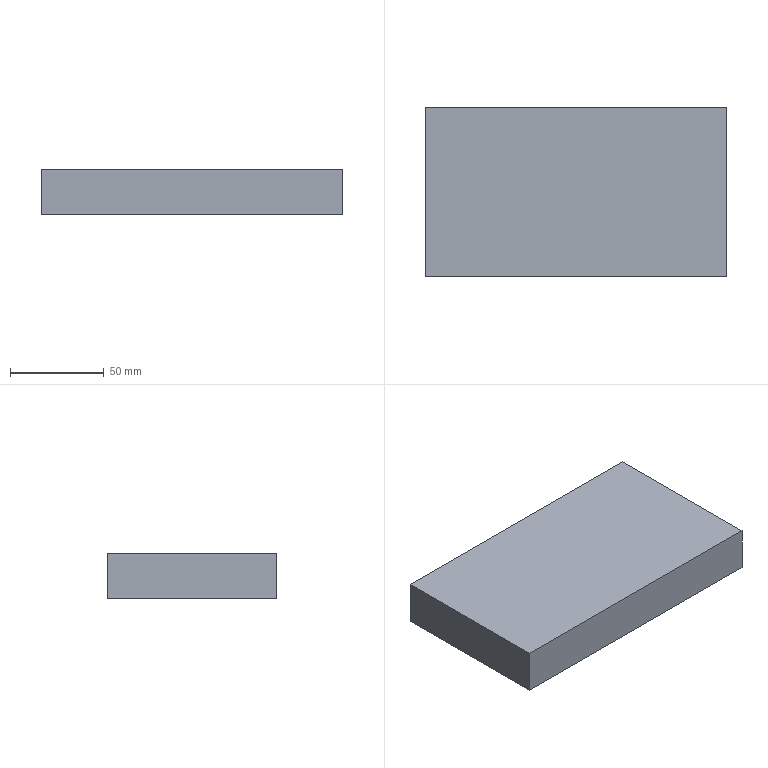Part | STEP file | 435_id754_x_t | 1 solid | 6 faces | box 160 x 90 x 24 mm | volume 345600 mm3 | plane 6
STEP:
#1=CARTESIAN_POINT('',(0.,0.,0.));
#2=DIRECTION('',(0.,0.,1.));
#3=DIRECTION('',(1.,0.,0.));
#4=AXIS2_PLACEMENT_3D('',#1,#2,#3);
#5=CARTESIAN_POINT('',(215.5,707.5,-3.997));
#6=VERTEX_POINT('',#5);
#7=CARTESIAN_POINT('',(375.5,707.5,-3.997));
#8=VERTEX_POINT('',#7);
#9=CARTESIAN_POINT('',(295.5,707.5,-3.997));
#10=DIRECTION('',(1.,0.,0.));
#11=VECTOR('',#10,1.);
#12=LINE('',#9,#11);
#13=CARTESIAN_POINT('',(295.5,752.5,-3.997));
#14=DIRECTION('',(0.,0.,1.));
#15=DIRECTION('',(1.,0.,0.));
#16=AXIS2_PLACEMENT_3D('',#13,#14,#15);
#17=PLANE('',#16);
#18=CARTESIAN_POINT('',(0.,-45.));
#19=DIRECTION('',(1.,0.));
#20=VECTOR('',#19,1.);
#21=LINE('',#18,#20);
#22=(GEOMETRIC_REPRESENTATION_CONTEXT(2)PARAMETRIC_REPRESENTATION_CONTEXT()REPRESENTATION_CONTEXT('',''));
#23=DEFINITIONAL_REPRESENTATION('',(#21),#22);
#24=PCURVE('',#17,#23);
#25=CARTESIAN_POINT('',(295.5,707.5,24.003));
#26=DIRECTION('',(0.,-1.,0.));
#27=DIRECTION('',(0.,0.,-1.));
#28=AXIS2_PLACEMENT_3D('',#25,#26,#27);
#29=PLANE('',#28);
#30=CARTESIAN_POINT('',(28.,0.));
#31=DIRECTION('',(0.,1.));
#32=VECTOR('',#31,1.);
#33=LINE('',#30,#32);
#34=(GEOMETRIC_REPRESENTATION_CONTEXT(2)PARAMETRIC_REPRESENTATION_CONTEXT()REPRESENTATION_CONTEXT('',''));
#35=DEFINITIONAL_REPRESENTATION('',(#33),#34);
#36=PCURVE('',#29,#35);
#37=SURFACE_CURVE('',#12,(#24,#36),.PCURVE_S1.);
#38=EDGE_CURVE('',#6,#8,#37,.T.);
#39=ORIENTED_EDGE('',*,*,#38,.F.);
#40=CARTESIAN_POINT('',(215.5,797.5,-3.997));
#41=VERTEX_POINT('',#40);
#42=CARTESIAN_POINT('',(215.5,752.5,-3.997));
#43=DIRECTION('',(0.,-1.,0.));
#44=VECTOR('',#43,1.);
#45=LINE('',#42,#44);
#46=CARTESIAN_POINT('',(-80.,0.));
#47=DIRECTION('',(0.,-1.));
#48=VECTOR('',#47,1.);
#49=LINE('',#46,#48);
#50=(GEOMETRIC_REPRESENTATION_CONTEXT(2)PARAMETRIC_REPRESENTATION_CONTEXT()REPRESENTATION_CONTEXT('',''));
#51=DEFINITIONAL_REPRESENTATION('',(#49),#50);
#52=PCURVE('',#17,#51);
#53=CARTESIAN_POINT('',(215.5,752.5,24.003));
#54=DIRECTION('',(-1.,0.,0.));
#55=DIRECTION('',(0.,0.,1.));
#56=AXIS2_PLACEMENT_3D('',#53,#54,#55);
#57=PLANE('',#56);
#58=CARTESIAN_POINT('',(-28.,0.));
#59=DIRECTION('',(0.,-1.));
#60=VECTOR('',#59,1.);
#61=LINE('',#58,#60);
#62=(GEOMETRIC_REPRESENTATION_CONTEXT(2)PARAMETRIC_REPRESENTATION_CONTEXT()REPRESENTATION_CONTEXT('',''));
#63=DEFINITIONAL_REPRESENTATION('',(#61),#62);
#64=PCURVE('',#57,#63);
#65=SURFACE_CURVE('',#45,(#52,#64),.PCURVE_S1.);
#66=EDGE_CURVE('',#41,#6,#65,.T.);
#67=ORIENTED_EDGE('',*,*,#66,.F.);
#68=CARTESIAN_POINT('',(375.5,797.5,-3.997));
#69=VERTEX_POINT('',#68);
#70=CARTESIAN_POINT('',(295.5,797.5,-3.997));
#71=DIRECTION('',(-1.,0.,0.));
#72=VECTOR('',#71,1.);
#73=LINE('',#70,#72);
#74=CARTESIAN_POINT('',(0.,45.));
#75=DIRECTION('',(-1.,0.));
#76=VECTOR('',#75,1.);
#77=LINE('',#74,#76);
#78=(GEOMETRIC_REPRESENTATION_CONTEXT(2)PARAMETRIC_REPRESENTATION_CONTEXT()REPRESENTATION_CONTEXT('',''));
#79=DEFINITIONAL_REPRESENTATION('',(#77),#78);
#80=PCURVE('',#17,#79);
#81=CARTESIAN_POINT('',(295.5,797.5,24.003));
#82=DIRECTION('',(0.,1.,0.));
#83=DIRECTION('',(0.,0.,1.));
#84=AXIS2_PLACEMENT_3D('',#81,#82,#83);
#85=PLANE('',#84);
#86=CARTESIAN_POINT('',(-28.,0.));
#87=DIRECTION('',(0.,-1.));
#88=VECTOR('',#87,1.);
#89=LINE('',#86,#88);
#90=(GEOMETRIC_REPRESENTATION_CONTEXT(2)PARAMETRIC_REPRESENTATION_CONTEXT()REPRESENTATION_CONTEXT('',''));
#91=DEFINITIONAL_REPRESENTATION('',(#89),#90);
#92=PCURVE('',#85,#91);
#93=SURFACE_CURVE('',#73,(#80,#92),.PCURVE_S1.);
#94=EDGE_CURVE('',#69,#41,#93,.T.);
#95=ORIENTED_EDGE('',*,*,#94,.F.);
#96=CARTESIAN_POINT('',(375.5,752.5,-3.997));
#97=DIRECTION('',(0.,1.,0.));
#98=VECTOR('',#97,1.);
#99=LINE('',#96,#98);
#100=CARTESIAN_POINT('',(80.,0.));
#101=DIRECTION('',(0.,1.));
#102=VECTOR('',#101,1.);
#103=LINE('',#100,#102);
#104=(GEOMETRIC_REPRESENTATION_CONTEXT(2)PARAMETRIC_REPRESENTATION_CONTEXT()REPRESENTATION_CONTEXT('',''));
#105=DEFINITIONAL_REPRESENTATION('',(#103),#104);
#106=PCURVE('',#17,#105);
#107=CARTESIAN_POINT('',(375.5,752.5,24.003));
#108=DIRECTION('',(1.,0.,0.));
#109=DIRECTION('',(0.,0.,-1.));
#110=AXIS2_PLACEMENT_3D('',#107,#108,#109);
#111=PLANE('',#110);
#112=CARTESIAN_POINT('',(28.,0.));
#113=DIRECTION('',(0.,1.));
#114=VECTOR('',#113,1.);
#115=LINE('',#112,#114);
#116=(GEOMETRIC_REPRESENTATION_CONTEXT(2)PARAMETRIC_REPRESENTATION_CONTEXT()REPRESENTATION_CONTEXT('',''));
#117=DEFINITIONAL_REPRESENTATION('',(#115),#116);
#118=PCURVE('',#111,#117);
#119=SURFACE_CURVE('',#99,(#106,#118),.PCURVE_S1.);
#120=EDGE_CURVE('',#8,#69,#119,.T.);
#121=ORIENTED_EDGE('',*,*,#120,.F.);
#122=EDGE_LOOP('',(#39,#67,#95,#121));
#123=FACE_BOUND('',#122,.T.);
#124=ADVANCED_FACE('',(#123),#17,.F.);
#125=CARTESIAN_POINT('',(215.5,707.5,20.003));
#126=VERTEX_POINT('',#125);
#127=CARTESIAN_POINT('',(215.5,707.5,24.003));
#128=DIRECTION('',(0.,0.,-1.));
#129=VECTOR('',#128,1.);
#130=LINE('',#127,#129);
#131=CARTESIAN_POINT('',(0.,-80.));
#132=DIRECTION('',(1.,0.));
#133=VECTOR('',#132,1.);
#134=LINE('',#131,#133);
#135=(GEOMETRIC_REPRESENTATION_CONTEXT(2)PARAMETRIC_REPRESENTATION_CONTEXT()REPRESENTATION_CONTEXT('',''));
#136=DEFINITIONAL_REPRESENTATION('',(#134),#135);
#137=PCURVE('',#29,#136);
#138=CARTESIAN_POINT('',(0.,-45.));
#139=DIRECTION('',(-1.,0.));
#140=VECTOR('',#139,1.);
#141=LINE('',#138,#140);
#142=(GEOMETRIC_REPRESENTATION_CONTEXT(2)PARAMETRIC_REPRESENTATION_CONTEXT()REPRESENTATION_CONTEXT('',''));
#143=DEFINITIONAL_REPRESENTATION('',(#141),#142);
#144=PCURVE('',#57,#143);
#145=SURFACE_CURVE('',#130,(#137,#144),.PCURVE_S1.);
#146=EDGE_CURVE('',#126,#6,#145,.T.);
#147=ORIENTED_EDGE('',*,*,#146,.T.);
#148=ORIENTED_EDGE('',*,*,#38,.T.);
#149=CARTESIAN_POINT('',(375.5,707.5,20.003));
#150=VERTEX_POINT('',#149);
#151=CARTESIAN_POINT('',(375.5,707.5,24.003));
#152=DIRECTION('',(0.,0.,-1.));
#153=VECTOR('',#152,1.);
#154=LINE('',#151,#153);
#155=CARTESIAN_POINT('',(0.,80.));
#156=DIRECTION('',(1.,0.));
#157=VECTOR('',#156,1.);
#158=LINE('',#155,#157);
#159=(GEOMETRIC_REPRESENTATION_CONTEXT(2)PARAMETRIC_REPRESENTATION_CONTEXT()REPRESENTATION_CONTEXT('',''));
#160=DEFINITIONAL_REPRESENTATION('',(#158),#159);
#161=PCURVE('',#29,#160);
#162=CARTESIAN_POINT('',(0.,-45.));
#163=DIRECTION('',(1.,0.));
#164=VECTOR('',#163,1.);
#165=LINE('',#162,#164);
#166=(GEOMETRIC_REPRESENTATION_CONTEXT(2)PARAMETRIC_REPRESENTATION_CONTEXT()REPRESENTATION_CONTEXT('',''));
#167=DEFINITIONAL_REPRESENTATION('',(#165),#166);
#168=PCURVE('',#111,#167);
#169=SURFACE_CURVE('',#154,(#161,#168),.PCURVE_S1.);
#170=EDGE_CURVE('',#150,#8,#169,.T.);
#171=ORIENTED_EDGE('',*,*,#170,.F.);
#172=CARTESIAN_POINT('',(295.5,707.5,20.003));
#173=DIRECTION('',(-1.,0.,0.));
#174=VECTOR('',#173,1.);
#175=LINE('',#172,#174);
#176=CARTESIAN_POINT('',(4.,0.));
#177=DIRECTION('',(0.,-1.));
#178=VECTOR('',#177,1.);
#179=LINE('',#176,#178);
#180=(GEOMETRIC_REPRESENTATION_CONTEXT(2)PARAMETRIC_REPRESENTATION_CONTEXT()REPRESENTATION_CONTEXT('',''));
#181=DEFINITIONAL_REPRESENTATION('',(#179),#180);
#182=PCURVE('',#29,#181);
#183=CARTESIAN_POINT('',(295.5,752.5,20.003));
#184=DIRECTION('',(0.,0.,1.));
#185=DIRECTION('',(1.,0.,0.));
#186=AXIS2_PLACEMENT_3D('',#183,#184,#185);
#187=PLANE('',#186);
#188=CARTESIAN_POINT('',(0.,-45.));
#189=DIRECTION('',(-1.,0.));
#190=VECTOR('',#189,1.);
#191=LINE('',#188,#190);
#192=(GEOMETRIC_REPRESENTATION_CONTEXT(2)PARAMETRIC_REPRESENTATION_CONTEXT()REPRESENTATION_CONTEXT('',''));
#193=DEFINITIONAL_REPRESENTATION('',(#191),#192);
#194=PCURVE('',#187,#193);
#195=SURFACE_CURVE('',#175,(#182,#194),.PCURVE_S1.);
#196=EDGE_CURVE('',#150,#126,#195,.T.);
#197=ORIENTED_EDGE('',*,*,#196,.T.);
#198=EDGE_LOOP('',(#147,#148,#171,#197));
#199=FACE_BOUND('',#198,.T.);
#200=ADVANCED_FACE('',(#199),#29,.T.);
#201=ORIENTED_EDGE('',*,*,#170,.T.);
#202=ORIENTED_EDGE('',*,*,#120,.T.);
#203=CARTESIAN_POINT('',(375.5,797.5,20.003));
#204=VERTEX_POINT('',#203);
#205=CARTESIAN_POINT('',(375.5,797.5,24.003));
#206=DIRECTION('',(0.,0.,-1.));
#207=VECTOR('',#206,1.);
#208=LINE('',#205,#207);
#209=CARTESIAN_POINT('',(0.,45.));
#210=DIRECTION('',(1.,0.));
#211=VECTOR('',#210,1.);
#212=LINE('',#209,#211);
#213=(GEOMETRIC_REPRESENTATION_CONTEXT(2)PARAMETRIC_REPRESENTATION_CONTEXT()REPRESENTATION_CONTEXT('',''));
#214=DEFINITIONAL_REPRESENTATION('',(#212),#213);
#215=PCURVE('',#111,#214);
#216=CARTESIAN_POINT('',(0.,80.));
#217=DIRECTION('',(-1.,0.));
#218=VECTOR('',#217,1.);
#219=LINE('',#216,#218);
#220=(GEOMETRIC_REPRESENTATION_CONTEXT(2)PARAMETRIC_REPRESENTATION_CONTEXT()REPRESENTATION_CONTEXT('',''));
#221=DEFINITIONAL_REPRESENTATION('',(#219),#220);
#222=PCURVE('',#85,#221);
#223=SURFACE_CURVE('',#208,(#215,#222),.PCURVE_S1.);
#224=EDGE_CURVE('',#204,#69,#223,.T.);
#225=ORIENTED_EDGE('',*,*,#224,.F.);
#226=CARTESIAN_POINT('',(375.5,752.5,20.003));
#227=DIRECTION('',(0.,-1.,0.));
#228=VECTOR('',#227,1.);
#229=LINE('',#226,#228);
#230=CARTESIAN_POINT('',(4.,0.));
#231=DIRECTION('',(0.,-1.));
#232=VECTOR('',#231,1.);
#233=LINE('',#230,#232);
#234=(GEOMETRIC_REPRESENTATION_CONTEXT(2)PARAMETRIC_REPRESENTATION_CONTEXT()REPRESENTATION_CONTEXT('',''));
#235=DEFINITIONAL_REPRESENTATION('',(#233),#234);
#236=PCURVE('',#111,#235);
#237=CARTESIAN_POINT('',(80.,0.));
#238=DIRECTION('',(0.,-1.));
#239=VECTOR('',#238,1.);
#240=LINE('',#237,#239);
#241=(GEOMETRIC_REPRESENTATION_CONTEXT(2)PARAMETRIC_REPRESENTATION_CONTEXT()REPRESENTATION_CONTEXT('',''));
#242=DEFINITIONAL_REPRESENTATION('',(#240),#241);
#243=PCURVE('',#187,#242);
#244=SURFACE_CURVE('',#229,(#236,#243),.PCURVE_S1.);
#245=EDGE_CURVE('',#204,#150,#244,.T.);
#246=ORIENTED_EDGE('',*,*,#245,.T.);
#247=EDGE_LOOP('',(#201,#202,#225,#246));
#248=FACE_BOUND('',#247,.T.);
#249=ADVANCED_FACE('',(#248),#111,.T.);
#250=ORIENTED_EDGE('',*,*,#224,.T.);
#251=ORIENTED_EDGE('',*,*,#94,.T.);
#252=CARTESIAN_POINT('',(215.5,797.5,20.003));
#253=VERTEX_POINT('',#252);
#254=CARTESIAN_POINT('',(215.5,797.5,24.003));
#255=DIRECTION('',(0.,0.,-1.));
#256=VECTOR('',#255,1.);
#257=LINE('',#254,#256);
#258=CARTESIAN_POINT('',(0.,-80.));
#259=DIRECTION('',(-1.,0.));
#260=VECTOR('',#259,1.);
#261=LINE('',#258,#260);
#262=(GEOMETRIC_REPRESENTATION_CONTEXT(2)PARAMETRIC_REPRESENTATION_CONTEXT()REPRESENTATION_CONTEXT('',''));
#263=DEFINITIONAL_REPRESENTATION('',(#261),#262);
#264=PCURVE('',#85,#263);
#265=CARTESIAN_POINT('',(0.,45.));
#266=DIRECTION('',(-1.,0.));
#267=VECTOR('',#266,1.);
#268=LINE('',#265,#267);
#269=(GEOMETRIC_REPRESENTATION_CONTEXT(2)PARAMETRIC_REPRESENTATION_CONTEXT()REPRESENTATION_CONTEXT('',''));
#270=DEFINITIONAL_REPRESENTATION('',(#268),#269);
#271=PCURVE('',#57,#270);
#272=SURFACE_CURVE('',#257,(#264,#271),.PCURVE_S1.);
#273=EDGE_CURVE('',#253,#41,#272,.T.);
#274=ORIENTED_EDGE('',*,*,#273,.F.);
#275=CARTESIAN_POINT('',(295.5,797.5,20.003));
#276=DIRECTION('',(1.,0.,0.));
#277=VECTOR('',#276,1.);
#278=LINE('',#275,#277);
#279=CARTESIAN_POINT('',(-4.,0.));
#280=DIRECTION('',(0.,1.));
#281=VECTOR('',#280,1.);
#282=LINE('',#279,#281);
#283=(GEOMETRIC_REPRESENTATION_CONTEXT(2)PARAMETRIC_REPRESENTATION_CONTEXT()REPRESENTATION_CONTEXT('',''));
#284=DEFINITIONAL_REPRESENTATION('',(#282),#283);
#285=PCURVE('',#85,#284);
#286=CARTESIAN_POINT('',(0.,45.));
#287=DIRECTION('',(1.,0.));
#288=VECTOR('',#287,1.);
#289=LINE('',#286,#288);
#290=(GEOMETRIC_REPRESENTATION_CONTEXT(2)PARAMETRIC_REPRESENTATION_CONTEXT()REPRESENTATION_CONTEXT('',''));
#291=DEFINITIONAL_REPRESENTATION('',(#289),#290);
#292=PCURVE('',#187,#291);
#293=SURFACE_CURVE('',#278,(#285,#292),.PCURVE_S1.);
#294=EDGE_CURVE('',#253,#204,#293,.T.);
#295=ORIENTED_EDGE('',*,*,#294,.T.);
#296=EDGE_LOOP('',(#250,#251,#274,#295));
#297=FACE_BOUND('',#296,.T.);
#298=ADVANCED_FACE('',(#297),#85,.T.);
#299=CARTESIAN_POINT('',(215.5,752.5,20.003));
#300=DIRECTION('',(0.,1.,0.));
#301=VECTOR('',#300,1.);
#302=LINE('',#299,#301);
#303=CARTESIAN_POINT('',(-80.,0.));
#304=DIRECTION('',(0.,1.));
#305=VECTOR('',#304,1.);
#306=LINE('',#303,#305);
#307=(GEOMETRIC_REPRESENTATION_CONTEXT(2)PARAMETRIC_REPRESENTATION_CONTEXT()REPRESENTATION_CONTEXT('',''));
#308=DEFINITIONAL_REPRESENTATION('',(#306),#307);
#309=PCURVE('',#187,#308);
#310=CARTESIAN_POINT('',(-4.,0.));
#311=DIRECTION('',(0.,1.));
#312=VECTOR('',#311,1.);
#313=LINE('',#310,#312);
#314=(GEOMETRIC_REPRESENTATION_CONTEXT(2)PARAMETRIC_REPRESENTATION_CONTEXT()REPRESENTATION_CONTEXT('',''));
#315=DEFINITIONAL_REPRESENTATION('',(#313),#314);
#316=PCURVE('',#57,#315);
#317=SURFACE_CURVE('',#302,(#309,#316),.PCURVE_S1.);
#318=EDGE_CURVE('',#126,#253,#317,.T.);
#319=ORIENTED_EDGE('',*,*,#318,.F.);
#320=ORIENTED_EDGE('',*,*,#196,.F.);
#321=ORIENTED_EDGE('',*,*,#245,.F.);
#322=ORIENTED_EDGE('',*,*,#294,.F.);
#323=EDGE_LOOP('',(#319,#320,#321,#322));
#324=FACE_BOUND('',#323,.T.);
#325=ADVANCED_FACE('',(#324),#187,.T.);
#326=ORIENTED_EDGE('',*,*,#318,.T.);
#327=ORIENTED_EDGE('',*,*,#273,.T.);
#328=ORIENTED_EDGE('',*,*,#66,.T.);
#329=ORIENTED_EDGE('',*,*,#146,.F.);
#330=EDGE_LOOP('',(#326,#327,#328,#329));
#331=FACE_BOUND('',#330,.T.);
#332=ADVANCED_FACE('',(#331),#57,.T.);
#333=CLOSED_SHELL('',(#124,#200,#249,#298,#325,#332));
#334=MANIFOLD_SOLID_BREP('',#333);
#335=(LENGTH_UNIT()NAMED_UNIT(*)SI_UNIT(.MILLI.,.METRE.));
#336=UNCERTAINTY_MEASURE_WITH_UNIT(LENGTH_MEASURE(0.0000001),#335,'','');
#337=(NAMED_UNIT(*)PLANE_ANGLE_UNIT()SI_UNIT($,.RADIAN.));
#338=(NAMED_UNIT(*)SI_UNIT($,.STERADIAN.)SOLID_ANGLE_UNIT());
#339=(GEOMETRIC_REPRESENTATION_CONTEXT(3)GLOBAL_UNCERTAINTY_ASSIGNED_CONTEXT((#336))GLOBAL_UNIT_ASSIGNED_CONTEXT((#335,#337,#338))REPRESENTATION_CONTEXT('',''));
#340=ADVANCED_BREP_SHAPE_REPRESENTATION('',(#4,#334),#339);